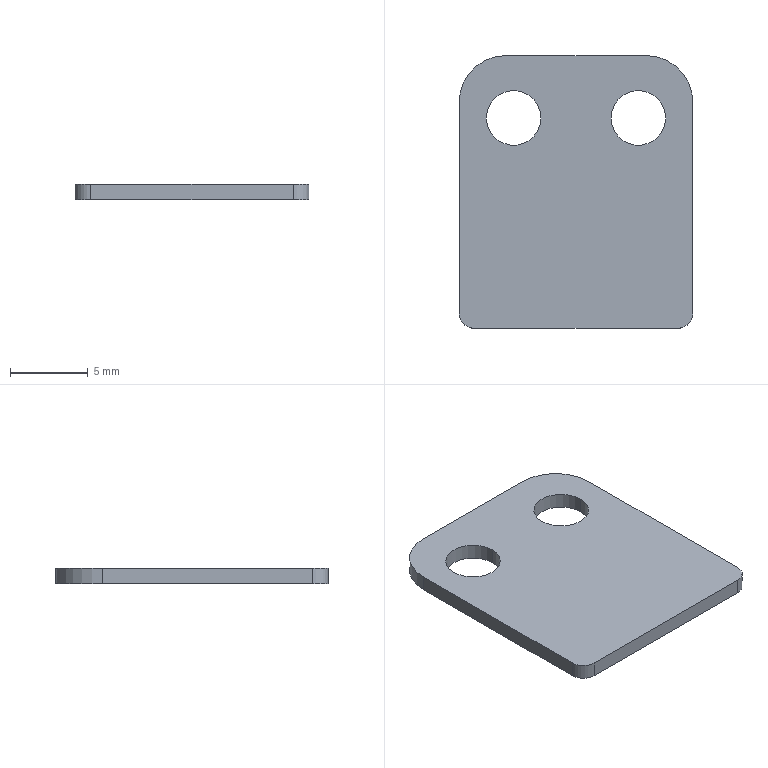Part | STEP file | LES120 homing stopper^FTH120-PD-direct-drive motor | 1 solid | 14 faces | box 15 x 17.5 x 1 mm | volume 238.966 mm3 | cylinder 8 | plane 6 | commonest cylinder face diameters 3.5 x4 2 x2 6 x2
STEP:
#1=CARTESIAN_POINT('',(-5.75,4.75,0.));
#2=VERTEX_POINT('',#1);
#3=CARTESIAN_POINT('',(-2.25,4.75,0.));
#4=VERTEX_POINT('',#3);
#5=CARTESIAN_POINT('',(-4.,4.75,0.));
#6=DIRECTION('',(0.,0.,1.));
#7=DIRECTION('',(1.,0.,0.));
#8=AXIS2_PLACEMENT_3D('',#5,#6,#7);
#9=CIRCLE('',#8,1.75);
#10=EDGE_CURVE('',#2,#4,#9,.T.);
#11=ORIENTED_EDGE('',*,*,#10,.F.);
#12=CARTESIAN_POINT('',(-5.75,4.75,1.));
#13=VERTEX_POINT('',#12);
#14=CARTESIAN_POINT('',(-5.75,4.75,0.));
#15=DIRECTION('',(0.,0.,1.));
#16=VECTOR('',#15,1000.);
#17=LINE('',#14,#16);
#18=EDGE_CURVE('',#2,#13,#17,.T.);
#19=ORIENTED_EDGE('',*,*,#18,.T.);
#20=CARTESIAN_POINT('',(-2.25,4.75,1.));
#21=VERTEX_POINT('',#20);
#22=CARTESIAN_POINT('',(-4.,4.75,1.));
#23=DIRECTION('',(0.,0.,1.));
#24=DIRECTION('',(1.,0.,0.));
#25=AXIS2_PLACEMENT_3D('',#22,#23,#24);
#26=CIRCLE('',#25,1.75);
#27=EDGE_CURVE('',#13,#21,#26,.T.);
#28=ORIENTED_EDGE('',*,*,#27,.T.);
#29=CARTESIAN_POINT('',(-2.25,4.75,0.));
#30=DIRECTION('',(0.,0.,1.));
#31=VECTOR('',#30,1000.);
#32=LINE('',#29,#31);
#33=EDGE_CURVE('',#4,#21,#32,.T.);
#34=ORIENTED_EDGE('',*,*,#33,.F.);
#35=EDGE_LOOP('',(#11,#19,#28,#34));
#36=FACE_OUTER_BOUND('',#35,.T.);
#37=CARTESIAN_POINT('',(-4.,4.75,0.));
#38=DIRECTION('',(0.,0.,1.));
#39=DIRECTION('',(1.,0.,0.));
#40=AXIS2_PLACEMENT_3D('',#37,#38,#39);
#41=CYLINDRICAL_SURFACE('',#40,1.75);
#42=ADVANCED_FACE('',(#36),#41,.F.);
#43=CARTESIAN_POINT('',(2.25,4.75,0.));
#44=VERTEX_POINT('',#43);
#45=CARTESIAN_POINT('',(5.75,4.75,0.));
#46=VERTEX_POINT('',#45);
#47=CARTESIAN_POINT('',(4.,4.75,0.));
#48=DIRECTION('',(0.,0.,1.));
#49=DIRECTION('',(1.,0.,0.));
#50=AXIS2_PLACEMENT_3D('',#47,#48,#49);
#51=CIRCLE('',#50,1.75);
#52=EDGE_CURVE('',#44,#46,#51,.T.);
#53=ORIENTED_EDGE('',*,*,#52,.F.);
#54=CARTESIAN_POINT('',(2.25,4.75,1.));
#55=VERTEX_POINT('',#54);
#56=CARTESIAN_POINT('',(2.25,4.75,0.));
#57=DIRECTION('',(0.,0.,1.));
#58=VECTOR('',#57,1000.);
#59=LINE('',#56,#58);
#60=EDGE_CURVE('',#44,#55,#59,.T.);
#61=ORIENTED_EDGE('',*,*,#60,.T.);
#62=CARTESIAN_POINT('',(5.75,4.75,1.));
#63=VERTEX_POINT('',#62);
#64=CARTESIAN_POINT('',(4.,4.75,1.));
#65=DIRECTION('',(0.,0.,1.));
#66=DIRECTION('',(1.,0.,0.));
#67=AXIS2_PLACEMENT_3D('',#64,#65,#66);
#68=CIRCLE('',#67,1.75);
#69=EDGE_CURVE('',#55,#63,#68,.T.);
#70=ORIENTED_EDGE('',*,*,#69,.T.);
#71=CARTESIAN_POINT('',(5.75,4.75,0.));
#72=DIRECTION('',(0.,0.,1.));
#73=VECTOR('',#72,1000.);
#74=LINE('',#71,#73);
#75=EDGE_CURVE('',#46,#63,#74,.T.);
#76=ORIENTED_EDGE('',*,*,#75,.F.);
#77=EDGE_LOOP('',(#53,#61,#70,#76));
#78=FACE_OUTER_BOUND('',#77,.T.);
#79=CARTESIAN_POINT('',(4.,4.75,0.));
#80=DIRECTION('',(0.,0.,1.));
#81=DIRECTION('',(1.,0.,0.));
#82=AXIS2_PLACEMENT_3D('',#79,#80,#81);
#83=CYLINDRICAL_SURFACE('',#82,1.75);
#84=ADVANCED_FACE('',(#78),#83,.F.);
#85=CARTESIAN_POINT('',(7.5,-7.75,1.));
#86=VERTEX_POINT('',#85);
#87=CARTESIAN_POINT('',(6.5,-8.75,1.));
#88=VERTEX_POINT('',#87);
#89=CARTESIAN_POINT('',(6.5,-7.75,1.));
#90=DIRECTION('',(0.,0.,-1.));
#91=DIRECTION('',(-1.,0.,0.));
#92=AXIS2_PLACEMENT_3D('',#89,#90,#91);
#93=CIRCLE('',#92,1.);
#94=EDGE_CURVE('',#86,#88,#93,.T.);
#95=ORIENTED_EDGE('',*,*,#94,.F.);
#96=CARTESIAN_POINT('',(7.5,5.75,1.));
#97=VERTEX_POINT('',#96);
#98=CARTESIAN_POINT('',(7.5,0.,1.));
#99=DIRECTION('',(0.,-1.,0.));
#100=VECTOR('',#99,1000.);
#101=LINE('',#98,#100);
#102=EDGE_CURVE('',#97,#86,#101,.T.);
#103=ORIENTED_EDGE('',*,*,#102,.F.);
#104=CARTESIAN_POINT('',(4.5,8.75,1.));
#105=VERTEX_POINT('',#104);
#106=CARTESIAN_POINT('',(4.5,5.75,1.));
#107=DIRECTION('',(0.,0.,-1.));
#108=DIRECTION('',(-1.,0.,0.));
#109=AXIS2_PLACEMENT_3D('',#106,#107,#108);
#110=CIRCLE('',#109,3.);
#111=EDGE_CURVE('',#105,#97,#110,.T.);
#112=ORIENTED_EDGE('',*,*,#111,.F.);
#113=CARTESIAN_POINT('',(-4.5,8.75,1.));
#114=VERTEX_POINT('',#113);
#115=CARTESIAN_POINT('',(0.,8.75,1.));
#116=DIRECTION('',(1.,0.,0.));
#117=VECTOR('',#116,1000.);
#118=LINE('',#115,#117);
#119=EDGE_CURVE('',#114,#105,#118,.T.);
#120=ORIENTED_EDGE('',*,*,#119,.F.);
#121=CARTESIAN_POINT('',(-7.5,5.75,1.));
#122=VERTEX_POINT('',#121);
#123=CARTESIAN_POINT('',(-4.5,5.75,1.));
#124=DIRECTION('',(0.,0.,-1.));
#125=DIRECTION('',(-1.,0.,0.));
#126=AXIS2_PLACEMENT_3D('',#123,#124,#125);
#127=CIRCLE('',#126,3.);
#128=EDGE_CURVE('',#122,#114,#127,.T.);
#129=ORIENTED_EDGE('',*,*,#128,.F.);
#130=CARTESIAN_POINT('',(-7.5,-7.75,1.));
#131=VERTEX_POINT('',#130);
#132=CARTESIAN_POINT('',(-7.5,0.,1.));
#133=DIRECTION('',(0.,1.,0.));
#134=VECTOR('',#133,1000.);
#135=LINE('',#132,#134);
#136=EDGE_CURVE('',#131,#122,#135,.T.);
#137=ORIENTED_EDGE('',*,*,#136,.F.);
#138=CARTESIAN_POINT('',(-6.5,-8.75,1.));
#139=VERTEX_POINT('',#138);
#140=CARTESIAN_POINT('',(-6.5,-7.75,1.));
#141=DIRECTION('',(0.,0.,-1.));
#142=DIRECTION('',(-1.,0.,0.));
#143=AXIS2_PLACEMENT_3D('',#140,#141,#142);
#144=CIRCLE('',#143,1.);
#145=EDGE_CURVE('',#139,#131,#144,.T.);
#146=ORIENTED_EDGE('',*,*,#145,.F.);
#147=CARTESIAN_POINT('',(0.,-8.75,1.));
#148=DIRECTION('',(-1.,0.,0.));
#149=VECTOR('',#148,1000.);
#150=LINE('',#147,#149);
#151=EDGE_CURVE('',#88,#139,#150,.T.);
#152=ORIENTED_EDGE('',*,*,#151,.F.);
#153=EDGE_LOOP('',(#95,#103,#112,#120,#129,#137,#146,#152));
#154=FACE_OUTER_BOUND('',#153,.T.);
#155=CARTESIAN_POINT('',(-4.,4.75,1.));
#156=DIRECTION('',(0.,0.,1.));
#157=DIRECTION('',(1.,0.,0.));
#158=AXIS2_PLACEMENT_3D('',#155,#156,#157);
#159=CIRCLE('',#158,1.75);
#160=EDGE_CURVE('',#21,#13,#159,.T.);
#161=ORIENTED_EDGE('',*,*,#160,.F.);
#162=ORIENTED_EDGE('',*,*,#27,.F.);
#163=EDGE_LOOP('',(#161,#162));
#164=FACE_BOUND('',#163,.T.);
#165=CARTESIAN_POINT('',(4.,4.75,1.));
#166=DIRECTION('',(0.,0.,1.));
#167=DIRECTION('',(1.,0.,0.));
#168=AXIS2_PLACEMENT_3D('',#165,#166,#167);
#169=CIRCLE('',#168,1.75);
#170=EDGE_CURVE('',#63,#55,#169,.T.);
#171=ORIENTED_EDGE('',*,*,#170,.F.);
#172=ORIENTED_EDGE('',*,*,#69,.F.);
#173=EDGE_LOOP('',(#171,#172));
#174=FACE_BOUND('',#173,.T.);
#175=CARTESIAN_POINT('',(0.,0.,1.));
#176=DIRECTION('',(0.,0.,-1.));
#177=DIRECTION('',(-1.,0.,0.));
#178=AXIS2_PLACEMENT_3D('',#175,#176,#177);
#179=PLANE('',#178);
#180=ADVANCED_FACE('',(#154,#164,#174),#179,.F.);
#181=CARTESIAN_POINT('',(6.5,-8.75,0.));
#182=VERTEX_POINT('',#181);
#183=CARTESIAN_POINT('',(6.5,-8.75,1.));
#184=DIRECTION('',(0.,0.,-1.));
#185=VECTOR('',#184,1000.);
#186=LINE('',#183,#185);
#187=EDGE_CURVE('',#88,#182,#186,.T.);
#188=ORIENTED_EDGE('',*,*,#187,.F.);
#189=ORIENTED_EDGE('',*,*,#151,.T.);
#190=CARTESIAN_POINT('',(-6.5,-8.75,0.));
#191=VERTEX_POINT('',#190);
#192=CARTESIAN_POINT('',(-6.5,-8.75,1.));
#193=DIRECTION('',(0.,0.,1.));
#194=VECTOR('',#193,1000.);
#195=LINE('',#192,#194);
#196=EDGE_CURVE('',#191,#139,#195,.T.);
#197=ORIENTED_EDGE('',*,*,#196,.F.);
#198=CARTESIAN_POINT('',(-7.5,-8.75,0.));
#199=DIRECTION('',(-1.,0.,0.));
#200=VECTOR('',#199,1000.);
#201=LINE('',#198,#200);
#202=EDGE_CURVE('',#182,#191,#201,.T.);
#203=ORIENTED_EDGE('',*,*,#202,.F.);
#204=EDGE_LOOP('',(#188,#189,#197,#203));
#205=FACE_OUTER_BOUND('',#204,.T.);
#206=CARTESIAN_POINT('',(-7.5,-8.75,1.));
#207=DIRECTION('',(0.,1.,0.));
#208=DIRECTION('',(0.,0.,1.));
#209=AXIS2_PLACEMENT_3D('',#206,#207,#208);
#210=PLANE('',#209);
#211=ADVANCED_FACE('',(#205),#210,.F.);
#212=CARTESIAN_POINT('',(7.5,-7.75,0.));
#213=VERTEX_POINT('',#212);
#214=CARTESIAN_POINT('',(6.5,-7.75,0.));
#215=DIRECTION('',(0.,0.,1.));
#216=DIRECTION('',(-1.,0.,0.));
#217=AXIS2_PLACEMENT_3D('',#214,#215,#216);
#218=CIRCLE('',#217,1.);
#219=EDGE_CURVE('',#182,#213,#218,.T.);
#220=ORIENTED_EDGE('',*,*,#219,.T.);
#221=CARTESIAN_POINT('',(7.5,-7.75,1.));
#222=DIRECTION('',(0.,0.,1.));
#223=VECTOR('',#222,1000.);
#224=LINE('',#221,#223);
#225=EDGE_CURVE('',#213,#86,#224,.T.);
#226=ORIENTED_EDGE('',*,*,#225,.T.);
#227=ORIENTED_EDGE('',*,*,#94,.T.);
#228=ORIENTED_EDGE('',*,*,#187,.T.);
#229=EDGE_LOOP('',(#220,#226,#227,#228));
#230=FACE_OUTER_BOUND('',#229,.T.);
#231=CARTESIAN_POINT('',(6.5,-7.75,1.));
#232=DIRECTION('',(0.,0.,-1.));
#233=DIRECTION('',(-1.,0.,0.));
#234=AXIS2_PLACEMENT_3D('',#231,#232,#233);
#235=CYLINDRICAL_SURFACE('',#234,1.);
#236=ADVANCED_FACE('',(#230),#235,.T.);
#237=ORIENTED_EDGE('',*,*,#225,.F.);
#238=CARTESIAN_POINT('',(7.5,5.75,0.));
#239=VERTEX_POINT('',#238);
#240=CARTESIAN_POINT('',(7.5,-8.75,0.));
#241=DIRECTION('',(0.,-1.,0.));
#242=VECTOR('',#241,1000.);
#243=LINE('',#240,#242);
#244=EDGE_CURVE('',#239,#213,#243,.T.);
#245=ORIENTED_EDGE('',*,*,#244,.F.);
#246=CARTESIAN_POINT('',(7.5,5.75,1.));
#247=DIRECTION('',(0.,0.,-1.));
#248=VECTOR('',#247,1000.);
#249=LINE('',#246,#248);
#250=EDGE_CURVE('',#97,#239,#249,.T.);
#251=ORIENTED_EDGE('',*,*,#250,.F.);
#252=ORIENTED_EDGE('',*,*,#102,.T.);
#253=EDGE_LOOP('',(#237,#245,#251,#252));
#254=FACE_OUTER_BOUND('',#253,.T.);
#255=CARTESIAN_POINT('',(7.5,-8.75,1.));
#256=DIRECTION('',(-1.,0.,0.));
#257=DIRECTION('',(0.,0.,1.));
#258=AXIS2_PLACEMENT_3D('',#255,#256,#257);
#259=PLANE('',#258);
#260=ADVANCED_FACE('',(#254),#259,.F.);
#261=CARTESIAN_POINT('',(4.5,8.75,0.));
#262=VERTEX_POINT('',#261);
#263=CARTESIAN_POINT('',(4.5,5.75,0.));
#264=DIRECTION('',(0.,0.,1.));
#265=DIRECTION('',(-1.,0.,0.));
#266=AXIS2_PLACEMENT_3D('',#263,#264,#265);
#267=CIRCLE('',#266,3.);
#268=EDGE_CURVE('',#239,#262,#267,.T.);
#269=ORIENTED_EDGE('',*,*,#268,.T.);
#270=CARTESIAN_POINT('',(4.5,8.75,1.));
#271=DIRECTION('',(0.,0.,1.));
#272=VECTOR('',#271,1000.);
#273=LINE('',#270,#272);
#274=EDGE_CURVE('',#262,#105,#273,.T.);
#275=ORIENTED_EDGE('',*,*,#274,.T.);
#276=ORIENTED_EDGE('',*,*,#111,.T.);
#277=ORIENTED_EDGE('',*,*,#250,.T.);
#278=EDGE_LOOP('',(#269,#275,#276,#277));
#279=FACE_OUTER_BOUND('',#278,.T.);
#280=CARTESIAN_POINT('',(4.5,5.75,1.));
#281=DIRECTION('',(0.,0.,-1.));
#282=DIRECTION('',(-1.,0.,0.));
#283=AXIS2_PLACEMENT_3D('',#280,#281,#282);
#284=CYLINDRICAL_SURFACE('',#283,3.);
#285=ADVANCED_FACE('',(#279),#284,.T.);
#286=ORIENTED_EDGE('',*,*,#274,.F.);
#287=CARTESIAN_POINT('',(-4.5,8.75,0.));
#288=VERTEX_POINT('',#287);
#289=CARTESIAN_POINT('',(-7.5,8.75,0.));
#290=DIRECTION('',(1.,0.,0.));
#291=VECTOR('',#290,1000.);
#292=LINE('',#289,#291);
#293=EDGE_CURVE('',#288,#262,#292,.T.);
#294=ORIENTED_EDGE('',*,*,#293,.F.);
#295=CARTESIAN_POINT('',(-4.5,8.75,1.));
#296=DIRECTION('',(0.,0.,-1.));
#297=VECTOR('',#296,1000.);
#298=LINE('',#295,#297);
#299=EDGE_CURVE('',#114,#288,#298,.T.);
#300=ORIENTED_EDGE('',*,*,#299,.F.);
#301=ORIENTED_EDGE('',*,*,#119,.T.);
#302=EDGE_LOOP('',(#286,#294,#300,#301));
#303=FACE_OUTER_BOUND('',#302,.T.);
#304=CARTESIAN_POINT('',(-7.5,8.75,1.));
#305=DIRECTION('',(0.,-1.,0.));
#306=DIRECTION('',(0.,0.,-1.));
#307=AXIS2_PLACEMENT_3D('',#304,#305,#306);
#308=PLANE('',#307);
#309=ADVANCED_FACE('',(#303),#308,.F.);
#310=CARTESIAN_POINT('',(-7.5,5.75,0.));
#311=VERTEX_POINT('',#310);
#312=CARTESIAN_POINT('',(-4.5,5.75,0.));
#313=DIRECTION('',(0.,0.,1.));
#314=DIRECTION('',(-1.,0.,0.));
#315=AXIS2_PLACEMENT_3D('',#312,#313,#314);
#316=CIRCLE('',#315,3.);
#317=EDGE_CURVE('',#288,#311,#316,.T.);
#318=ORIENTED_EDGE('',*,*,#317,.T.);
#319=CARTESIAN_POINT('',(-7.5,5.75,1.));
#320=DIRECTION('',(0.,0.,1.));
#321=VECTOR('',#320,1000.);
#322=LINE('',#319,#321);
#323=EDGE_CURVE('',#311,#122,#322,.T.);
#324=ORIENTED_EDGE('',*,*,#323,.T.);
#325=ORIENTED_EDGE('',*,*,#128,.T.);
#326=ORIENTED_EDGE('',*,*,#299,.T.);
#327=EDGE_LOOP('',(#318,#324,#325,#326));
#328=FACE_OUTER_BOUND('',#327,.T.);
#329=CARTESIAN_POINT('',(-4.5,5.75,1.));
#330=DIRECTION('',(0.,0.,-1.));
#331=DIRECTION('',(-1.,0.,0.));
#332=AXIS2_PLACEMENT_3D('',#329,#330,#331);
#333=CYLINDRICAL_SURFACE('',#332,3.);
#334=ADVANCED_FACE('',(#328),#333,.T.);
#335=CARTESIAN_POINT('',(-7.5,-7.75,0.));
#336=VERTEX_POINT('',#335);
#337=CARTESIAN_POINT('',(-7.5,-7.75,1.));
#338=DIRECTION('',(0.,0.,-1.));
#339=VECTOR('',#338,1000.);
#340=LINE('',#337,#339);
#341=EDGE_CURVE('',#131,#336,#340,.T.);
#342=ORIENTED_EDGE('',*,*,#341,.F.);
#343=ORIENTED_EDGE('',*,*,#136,.T.);
#344=ORIENTED_EDGE('',*,*,#323,.F.);
#345=CARTESIAN_POINT('',(-7.5,-8.75,0.));
#346=DIRECTION('',(0.,1.,0.));
#347=VECTOR('',#346,1000.);
#348=LINE('',#345,#347);
#349=EDGE_CURVE('',#336,#311,#348,.T.);
#350=ORIENTED_EDGE('',*,*,#349,.F.);
#351=EDGE_LOOP('',(#342,#343,#344,#350));
#352=FACE_OUTER_BOUND('',#351,.T.);
#353=CARTESIAN_POINT('',(-7.5,-8.75,1.));
#354=DIRECTION('',(1.,0.,0.));
#355=DIRECTION('',(0.,0.,-1.));
#356=AXIS2_PLACEMENT_3D('',#353,#354,#355);
#357=PLANE('',#356);
#358=ADVANCED_FACE('',(#352),#357,.F.);
#359=CARTESIAN_POINT('',(-6.5,-7.75,0.));
#360=DIRECTION('',(0.,0.,1.));
#361=DIRECTION('',(-1.,0.,0.));
#362=AXIS2_PLACEMENT_3D('',#359,#360,#361);
#363=CIRCLE('',#362,1.);
#364=EDGE_CURVE('',#336,#191,#363,.T.);
#365=ORIENTED_EDGE('',*,*,#364,.T.);
#366=ORIENTED_EDGE('',*,*,#196,.T.);
#367=ORIENTED_EDGE('',*,*,#145,.T.);
#368=ORIENTED_EDGE('',*,*,#341,.T.);
#369=EDGE_LOOP('',(#365,#366,#367,#368));
#370=FACE_OUTER_BOUND('',#369,.T.);
#371=CARTESIAN_POINT('',(-6.5,-7.75,1.));
#372=DIRECTION('',(0.,0.,-1.));
#373=DIRECTION('',(-1.,0.,0.));
#374=AXIS2_PLACEMENT_3D('',#371,#372,#373);
#375=CYLINDRICAL_SURFACE('',#374,1.);
#376=ADVANCED_FACE('',(#370),#375,.T.);
#377=ORIENTED_EDGE('',*,*,#18,.F.);
#378=CARTESIAN_POINT('',(-4.,4.75,0.));
#379=DIRECTION('',(0.,0.,1.));
#380=DIRECTION('',(1.,0.,0.));
#381=AXIS2_PLACEMENT_3D('',#378,#379,#380);
#382=CIRCLE('',#381,1.75);
#383=EDGE_CURVE('',#4,#2,#382,.T.);
#384=ORIENTED_EDGE('',*,*,#383,.F.);
#385=ORIENTED_EDGE('',*,*,#33,.T.);
#386=ORIENTED_EDGE('',*,*,#160,.T.);
#387=EDGE_LOOP('',(#377,#384,#385,#386));
#388=FACE_OUTER_BOUND('',#387,.T.);
#389=CARTESIAN_POINT('',(-4.,4.75,0.));
#390=DIRECTION('',(0.,0.,1.));
#391=DIRECTION('',(1.,0.,0.));
#392=AXIS2_PLACEMENT_3D('',#389,#390,#391);
#393=CYLINDRICAL_SURFACE('',#392,1.75);
#394=ADVANCED_FACE('',(#388),#393,.F.);
#395=ORIENTED_EDGE('',*,*,#60,.F.);
#396=CARTESIAN_POINT('',(4.,4.75,0.));
#397=DIRECTION('',(0.,0.,1.));
#398=DIRECTION('',(1.,0.,0.));
#399=AXIS2_PLACEMENT_3D('',#396,#397,#398);
#400=CIRCLE('',#399,1.75);
#401=EDGE_CURVE('',#46,#44,#400,.T.);
#402=ORIENTED_EDGE('',*,*,#401,.F.);
#403=ORIENTED_EDGE('',*,*,#75,.T.);
#404=ORIENTED_EDGE('',*,*,#170,.T.);
#405=EDGE_LOOP('',(#395,#402,#403,#404));
#406=FACE_OUTER_BOUND('',#405,.T.);
#407=CARTESIAN_POINT('',(4.,4.75,0.));
#408=DIRECTION('',(0.,0.,1.));
#409=DIRECTION('',(1.,0.,0.));
#410=AXIS2_PLACEMENT_3D('',#407,#408,#409);
#411=CYLINDRICAL_SURFACE('',#410,1.75);
#412=ADVANCED_FACE('',(#406),#411,.F.);
#413=ORIENTED_EDGE('',*,*,#293,.T.);
#414=ORIENTED_EDGE('',*,*,#268,.F.);
#415=ORIENTED_EDGE('',*,*,#244,.T.);
#416=ORIENTED_EDGE('',*,*,#219,.F.);
#417=ORIENTED_EDGE('',*,*,#202,.T.);
#418=ORIENTED_EDGE('',*,*,#364,.F.);
#419=ORIENTED_EDGE('',*,*,#349,.T.);
#420=ORIENTED_EDGE('',*,*,#317,.F.);
#421=EDGE_LOOP('',(#413,#414,#415,#416,#417,#418,#419,#420));
#422=FACE_OUTER_BOUND('',#421,.T.);
#423=ORIENTED_EDGE('',*,*,#383,.T.);
#424=ORIENTED_EDGE('',*,*,#10,.T.);
#425=EDGE_LOOP('',(#423,#424));
#426=FACE_BOUND('',#425,.T.);
#427=ORIENTED_EDGE('',*,*,#401,.T.);
#428=ORIENTED_EDGE('',*,*,#52,.T.);
#429=EDGE_LOOP('',(#427,#428));
#430=FACE_BOUND('',#429,.T.);
#431=CARTESIAN_POINT('',(0.,0.,0.));
#432=DIRECTION('',(0.,0.,-1.));
#433=DIRECTION('',(-1.,0.,0.));
#434=AXIS2_PLACEMENT_3D('',#431,#432,#433);
#435=PLANE('',#434);
#436=ADVANCED_FACE('',(#422,#426,#430),#435,.T.);
#437=CLOSED_SHELL('',(#42,#84,#180,#211,#236,#260,#285,#309,#334,#358,#376,#394,#412,#436));
#438=MANIFOLD_SOLID_BREP('',#437);
#439=CARTESIAN_POINT('',(0.,0.,0.));
#440=DIRECTION('',(0.,0.,1.));
#441=DIRECTION('',(1.,0.,0.));
#442=AXIS2_PLACEMENT_3D('',#439,#440,#441);
#443=(LENGTH_UNIT()NAMED_UNIT(*)SI_UNIT(.MILLI.,.METRE.));
#444=UNCERTAINTY_MEASURE_WITH_UNIT(LENGTH_MEASURE(0.00001),#443,'','');
#445=(NAMED_UNIT(*)PLANE_ANGLE_UNIT()SI_UNIT($,.RADIAN.));
#446=(NAMED_UNIT(*)SI_UNIT($,.STERADIAN.)SOLID_ANGLE_UNIT());
#447=(GEOMETRIC_REPRESENTATION_CONTEXT(3)GLOBAL_UNCERTAINTY_ASSIGNED_CONTEXT((#444))GLOBAL_UNIT_ASSIGNED_CONTEXT((#443,#445,#446))REPRESENTATION_CONTEXT('',''));
#448=ADVANCED_BREP_SHAPE_REPRESENTATION('',(#438,#442),#447);